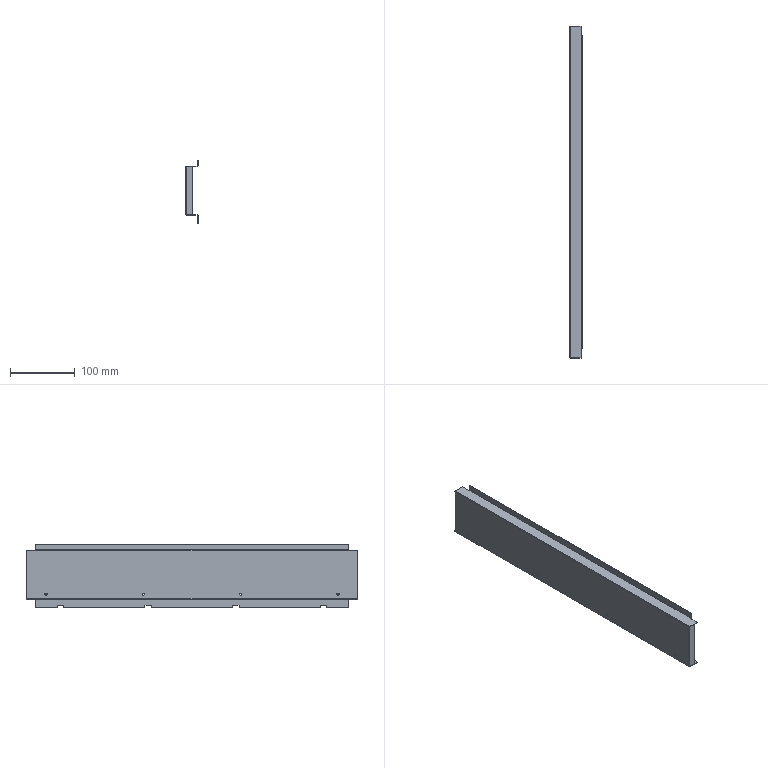Part | STEP file | 1 solid | 90 faces | box 18.5 x 511.5 x 98.4 mm | volume 54675 mm3 | plane 70 | cylinder 20 | commonest cylinder face diameters 3.3 x8 0.4 x6 2 x6